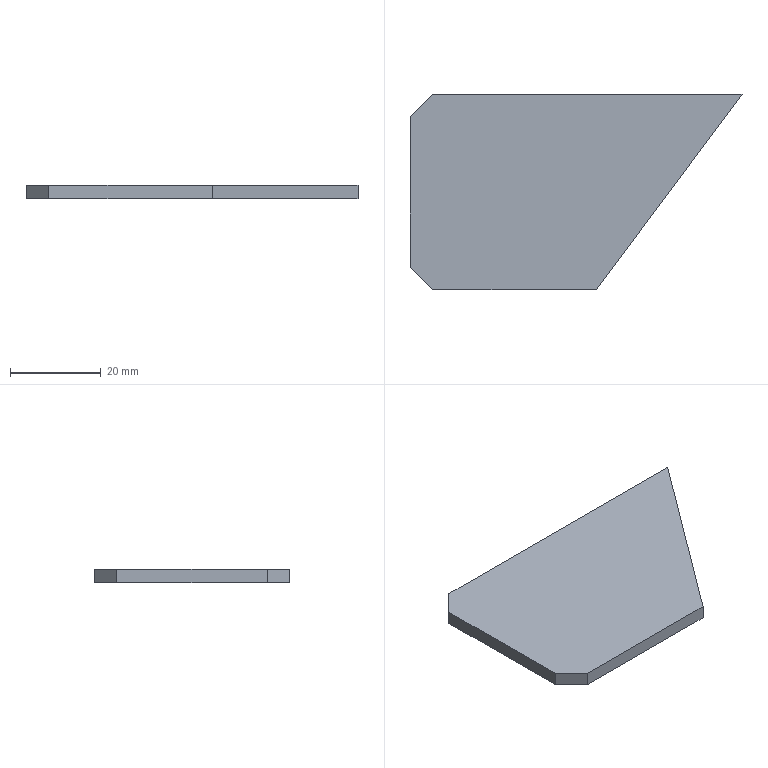Part | SolidWorks | features Chamfer 1, FlatPattern 1, ICE 1, SMBaseFlange 1, SheetMetal 1 | 1 solid | 8 faces | box 73 x 43 x 3 mm | volume 7278 mm3 | plane 8
STEP:
#1=CARTESIAN_POINT('',(73.,21.5,-3.));
#2=VERTEX_POINT('',#1);
#3=CARTESIAN_POINT('',(5.,21.5,-3.));
#4=VERTEX_POINT('',#3);
#5=CARTESIAN_POINT('',(73.,21.5,-3.));
#6=DIRECTION('',(-1.,0.,0.));
#7=VECTOR('',#6,1000.);
#8=LINE('',#5,#7);
#9=EDGE_CURVE('',#2,#4,#8,.T.);
#10=ORIENTED_EDGE('',*,*,#9,.T.);
#11=CARTESIAN_POINT('',(5.,21.5,0.));
#12=VERTEX_POINT('',#11);
#13=CARTESIAN_POINT('',(5.,21.5,-3.));
#14=DIRECTION('',(0.,0.,1.));
#15=VECTOR('',#14,1000.);
#16=LINE('',#13,#15);
#17=EDGE_CURVE('',#4,#12,#16,.T.);
#18=ORIENTED_EDGE('',*,*,#17,.T.);
#19=CARTESIAN_POINT('',(73.,21.5,0.));
#20=VERTEX_POINT('',#19);
#21=CARTESIAN_POINT('',(73.,21.5,0.));
#22=DIRECTION('',(-1.,0.,0.));
#23=VECTOR('',#22,1000.);
#24=LINE('',#21,#23);
#25=EDGE_CURVE('',#20,#12,#24,.T.);
#26=ORIENTED_EDGE('',*,*,#25,.F.);
#27=CARTESIAN_POINT('',(73.,21.5,-3.));
#28=DIRECTION('',(0.,0.,1.));
#29=VECTOR('',#28,1000.);
#30=LINE('',#27,#29);
#31=EDGE_CURVE('',#2,#20,#30,.T.);
#32=ORIENTED_EDGE('',*,*,#31,.F.);
#33=EDGE_LOOP('',(#10,#18,#26,#32));
#34=FACE_OUTER_BOUND('',#33,.T.);
#35=CARTESIAN_POINT('',(73.,21.5,-3.));
#36=DIRECTION('',(0.,1.,0.));
#37=DIRECTION('',(0.,0.,1.));
#38=AXIS2_PLACEMENT_3D('',#35,#36,#37);
#39=PLANE('',#38);
#40=ADVANCED_FACE('',(#34),#39,.T.);
#41=CARTESIAN_POINT('',(41.,-21.5,0.));
#42=VERTEX_POINT('',#41);
#43=CARTESIAN_POINT('',(41.,-21.5,0.));
#44=DIRECTION('',(0.597,0.8022,0.));
#45=VECTOR('',#44,1000.);
#46=LINE('',#43,#45);
#47=EDGE_CURVE('',#42,#20,#46,.T.);
#48=ORIENTED_EDGE('',*,*,#47,.F.);
#49=CARTESIAN_POINT('',(41.,-21.5,-3.));
#50=VERTEX_POINT('',#49);
#51=CARTESIAN_POINT('',(41.,-21.5,-3.));
#52=DIRECTION('',(0.,0.,1.));
#53=VECTOR('',#52,1000.);
#54=LINE('',#51,#53);
#55=EDGE_CURVE('',#50,#42,#54,.T.);
#56=ORIENTED_EDGE('',*,*,#55,.F.);
#57=CARTESIAN_POINT('',(41.,-21.5,-3.));
#58=DIRECTION('',(0.597,0.8022,0.));
#59=VECTOR('',#58,1000.);
#60=LINE('',#57,#59);
#61=EDGE_CURVE('',#50,#2,#60,.T.);
#62=ORIENTED_EDGE('',*,*,#61,.T.);
#63=ORIENTED_EDGE('',*,*,#31,.T.);
#64=EDGE_LOOP('',(#48,#56,#62,#63));
#65=FACE_OUTER_BOUND('',#64,.T.);
#66=CARTESIAN_POINT('',(41.,-21.5,-3.));
#67=DIRECTION('',(0.8022,-0.597,0.));
#68=DIRECTION('',(0.597,0.8022,0.));
#69=AXIS2_PLACEMENT_3D('',#66,#67,#68);
#70=PLANE('',#69);
#71=ADVANCED_FACE('',(#65),#70,.T.);
#72=CARTESIAN_POINT('',(5.,-21.5,0.));
#73=VERTEX_POINT('',#72);
#74=CARTESIAN_POINT('',(0.,-21.5,0.));
#75=DIRECTION('',(1.,0.,0.));
#76=VECTOR('',#75,1000.);
#77=LINE('',#74,#76);
#78=EDGE_CURVE('',#73,#42,#77,.T.);
#79=ORIENTED_EDGE('',*,*,#78,.F.);
#80=CARTESIAN_POINT('',(5.,-21.5,-3.));
#81=VERTEX_POINT('',#80);
#82=CARTESIAN_POINT('',(5.,-21.5,-3.));
#83=DIRECTION('',(0.,0.,-1.));
#84=VECTOR('',#83,1000.);
#85=LINE('',#82,#84);
#86=EDGE_CURVE('',#73,#81,#85,.T.);
#87=ORIENTED_EDGE('',*,*,#86,.T.);
#88=CARTESIAN_POINT('',(0.,-21.5,-3.));
#89=DIRECTION('',(1.,0.,0.));
#90=VECTOR('',#89,1000.);
#91=LINE('',#88,#90);
#92=EDGE_CURVE('',#81,#50,#91,.T.);
#93=ORIENTED_EDGE('',*,*,#92,.T.);
#94=ORIENTED_EDGE('',*,*,#55,.T.);
#95=EDGE_LOOP('',(#79,#87,#93,#94));
#96=FACE_OUTER_BOUND('',#95,.T.);
#97=CARTESIAN_POINT('',(0.,-21.5,-3.));
#98=DIRECTION('',(0.,-1.,0.));
#99=DIRECTION('',(0.,0.,-1.));
#100=AXIS2_PLACEMENT_3D('',#97,#98,#99);
#101=PLANE('',#100);
#102=ADVANCED_FACE('',(#96),#101,.T.);
#103=CARTESIAN_POINT('',(0.,16.5,-3.));
#104=VERTEX_POINT('',#103);
#105=CARTESIAN_POINT('',(0.,-16.5,-3.));
#106=VERTEX_POINT('',#105);
#107=CARTESIAN_POINT('',(0.,21.5,-3.));
#108=DIRECTION('',(0.,-1.,0.));
#109=VECTOR('',#108,1000.);
#110=LINE('',#107,#109);
#111=EDGE_CURVE('',#104,#106,#110,.T.);
#112=ORIENTED_EDGE('',*,*,#111,.T.);
#113=CARTESIAN_POINT('',(0.,-16.5,0.));
#114=VERTEX_POINT('',#113);
#115=CARTESIAN_POINT('',(0.,-16.5,-3.));
#116=DIRECTION('',(0.,0.,1.));
#117=VECTOR('',#116,1000.);
#118=LINE('',#115,#117);
#119=EDGE_CURVE('',#106,#114,#118,.T.);
#120=ORIENTED_EDGE('',*,*,#119,.T.);
#121=CARTESIAN_POINT('',(0.,16.5,0.));
#122=VERTEX_POINT('',#121);
#123=CARTESIAN_POINT('',(0.,21.5,0.));
#124=DIRECTION('',(0.,-1.,0.));
#125=VECTOR('',#124,1000.);
#126=LINE('',#123,#125);
#127=EDGE_CURVE('',#122,#114,#126,.T.);
#128=ORIENTED_EDGE('',*,*,#127,.F.);
#129=CARTESIAN_POINT('',(0.,16.5,-3.));
#130=DIRECTION('',(0.,0.,-1.));
#131=VECTOR('',#130,1000.);
#132=LINE('',#129,#131);
#133=EDGE_CURVE('',#122,#104,#132,.T.);
#134=ORIENTED_EDGE('',*,*,#133,.T.);
#135=EDGE_LOOP('',(#112,#120,#128,#134));
#136=FACE_OUTER_BOUND('',#135,.T.);
#137=CARTESIAN_POINT('',(0.,21.5,-3.));
#138=DIRECTION('',(-1.,0.,0.));
#139=DIRECTION('',(0.,-1.,0.));
#140=AXIS2_PLACEMENT_3D('',#137,#138,#139);
#141=PLANE('',#140);
#142=ADVANCED_FACE('',(#136),#141,.T.);
#143=ORIENTED_EDGE('',*,*,#92,.F.);
#144=CARTESIAN_POINT('',(0.,-16.5,-3.));
#145=DIRECTION('',(-0.7071,0.7071,0.));
#146=VECTOR('',#145,1000.);
#147=LINE('',#144,#146);
#148=EDGE_CURVE('',#81,#106,#147,.T.);
#149=ORIENTED_EDGE('',*,*,#148,.T.);
#150=ORIENTED_EDGE('',*,*,#111,.F.);
#151=CARTESIAN_POINT('',(5.,21.5,-3.));
#152=DIRECTION('',(0.7071,0.7071,0.));
#153=VECTOR('',#152,1000.);
#154=LINE('',#151,#153);
#155=EDGE_CURVE('',#104,#4,#154,.T.);
#156=ORIENTED_EDGE('',*,*,#155,.T.);
#157=ORIENTED_EDGE('',*,*,#9,.F.);
#158=ORIENTED_EDGE('',*,*,#61,.F.);
#159=EDGE_LOOP('',(#143,#149,#150,#156,#157,#158));
#160=FACE_OUTER_BOUND('',#159,.T.);
#161=CARTESIAN_POINT('',(0.,0.,-3.));
#162=DIRECTION('',(0.,0.,1.));
#163=DIRECTION('',(1.,0.,0.));
#164=AXIS2_PLACEMENT_3D('',#161,#162,#163);
#165=PLANE('',#164);
#166=ADVANCED_FACE('',(#160),#165,.F.);
#167=ORIENTED_EDGE('',*,*,#127,.T.);
#168=CARTESIAN_POINT('',(-8.25,-8.25,0.));
#169=DIRECTION('',(0.7071,-0.7071,0.));
#170=VECTOR('',#169,1000.);
#171=LINE('',#168,#170);
#172=EDGE_CURVE('',#114,#73,#171,.T.);
#173=ORIENTED_EDGE('',*,*,#172,.T.);
#174=ORIENTED_EDGE('',*,*,#78,.T.);
#175=ORIENTED_EDGE('',*,*,#47,.T.);
#176=ORIENTED_EDGE('',*,*,#25,.T.);
#177=CARTESIAN_POINT('',(-8.25,8.25,0.));
#178=DIRECTION('',(-0.7071,-0.7071,0.));
#179=VECTOR('',#178,1000.);
#180=LINE('',#177,#179);
#181=EDGE_CURVE('',#12,#122,#180,.T.);
#182=ORIENTED_EDGE('',*,*,#181,.T.);
#183=EDGE_LOOP('',(#167,#173,#174,#175,#176,#182));
#184=FACE_OUTER_BOUND('',#183,.T.);
#185=CARTESIAN_POINT('',(0.,0.,0.));
#186=DIRECTION('',(0.,0.,1.));
#187=DIRECTION('',(1.,0.,0.));
#188=AXIS2_PLACEMENT_3D('',#185,#186,#187);
#189=PLANE('',#188);
#190=ADVANCED_FACE('',(#184),#189,.T.);
#191=ORIENTED_EDGE('',*,*,#148,.F.);
#192=ORIENTED_EDGE('',*,*,#86,.F.);
#193=ORIENTED_EDGE('',*,*,#172,.F.);
#194=ORIENTED_EDGE('',*,*,#119,.F.);
#195=EDGE_LOOP('',(#191,#192,#193,#194));
#196=FACE_OUTER_BOUND('',#195,.T.);
#197=CARTESIAN_POINT('',(0.,-16.5,-3.));
#198=DIRECTION('',(0.7071,0.7071,0.));
#199=DIRECTION('',(0.,0.,1.));
#200=AXIS2_PLACEMENT_3D('',#197,#198,#199);
#201=PLANE('',#200);
#202=ADVANCED_FACE('',(#196),#201,.F.);
#203=ORIENTED_EDGE('',*,*,#155,.F.);
#204=ORIENTED_EDGE('',*,*,#133,.F.);
#205=ORIENTED_EDGE('',*,*,#181,.F.);
#206=ORIENTED_EDGE('',*,*,#17,.F.);
#207=EDGE_LOOP('',(#203,#204,#205,#206));
#208=FACE_OUTER_BOUND('',#207,.T.);
#209=CARTESIAN_POINT('',(5.,21.5,-3.));
#210=DIRECTION('',(0.7071,-0.7071,0.));
#211=DIRECTION('',(0.,0.,1.));
#212=AXIS2_PLACEMENT_3D('',#209,#210,#211);
#213=PLANE('',#212);
#214=ADVANCED_FACE('',(#208),#213,.F.);
#215=CLOSED_SHELL('',(#40,#71,#102,#142,#166,#190,#202,#214));
#216=MANIFOLD_SOLID_BREP('',#215);
#217=CARTESIAN_POINT('',(0.,0.,0.));
#218=DIRECTION('',(0.,0.,1.));
#219=DIRECTION('',(1.,0.,0.));
#220=AXIS2_PLACEMENT_3D('',#217,#218,#219);
#221=(LENGTH_UNIT()NAMED_UNIT(*)SI_UNIT(.MILLI.,.METRE.));
#222=UNCERTAINTY_MEASURE_WITH_UNIT(LENGTH_MEASURE(0.00001),#221,'','');
#223=(NAMED_UNIT(*)PLANE_ANGLE_UNIT()SI_UNIT($,.RADIAN.));
#224=(NAMED_UNIT(*)SI_UNIT($,.STERADIAN.)SOLID_ANGLE_UNIT());
#225=(GEOMETRIC_REPRESENTATION_CONTEXT(3)GLOBAL_UNCERTAINTY_ASSIGNED_CONTEXT((#222))GLOBAL_UNIT_ASSIGNED_CONTEXT((#221,#223,#224))REPRESENTATION_CONTEXT('',''));
#226=ADVANCED_BREP_SHAPE_REPRESENTATION('',(#216,#220),#225);